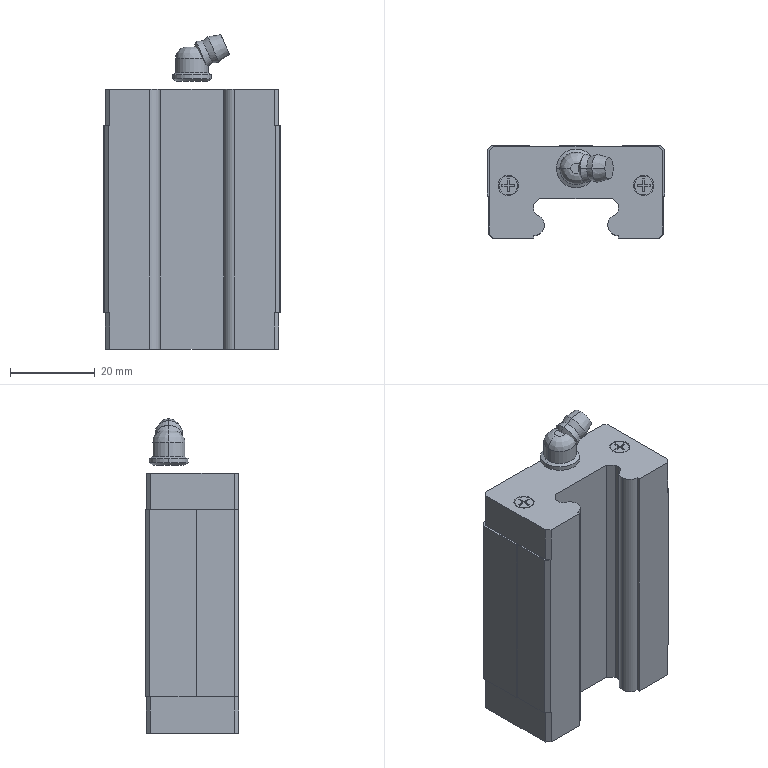Part | STEP file | block_SXRB28 | 3 solids | 185 faces | box 42 x 22 x 74.3 mm | volume 45231 mm3 | plane 102 | cylinder 53 | cone 28 | other 2 | commonest cylinder face diameters 3.08 x20 4.134 x8 4.4 x8 4.8 x8 5 x3 3 x2